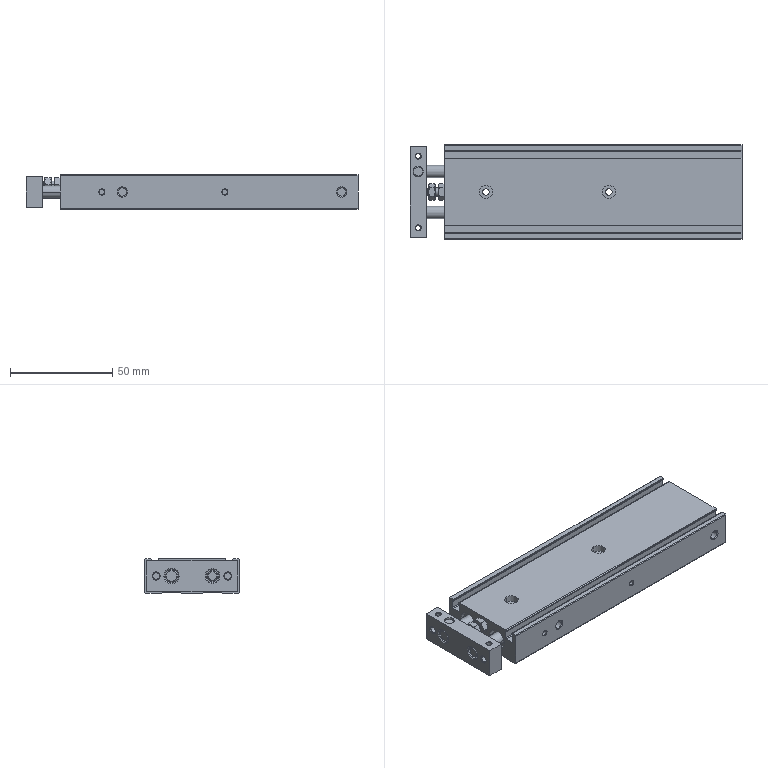Part | STEP file | 2 solids | 251 faces | box 162 x 46 x 17 mm | volume 100812 mm3 | cylinder 94 | plane 81 | cone 76 | commonest cylinder face diameters 2.459 x16 10 x16 0.8 x12 6 x10 3.242 x8 4.134 x8